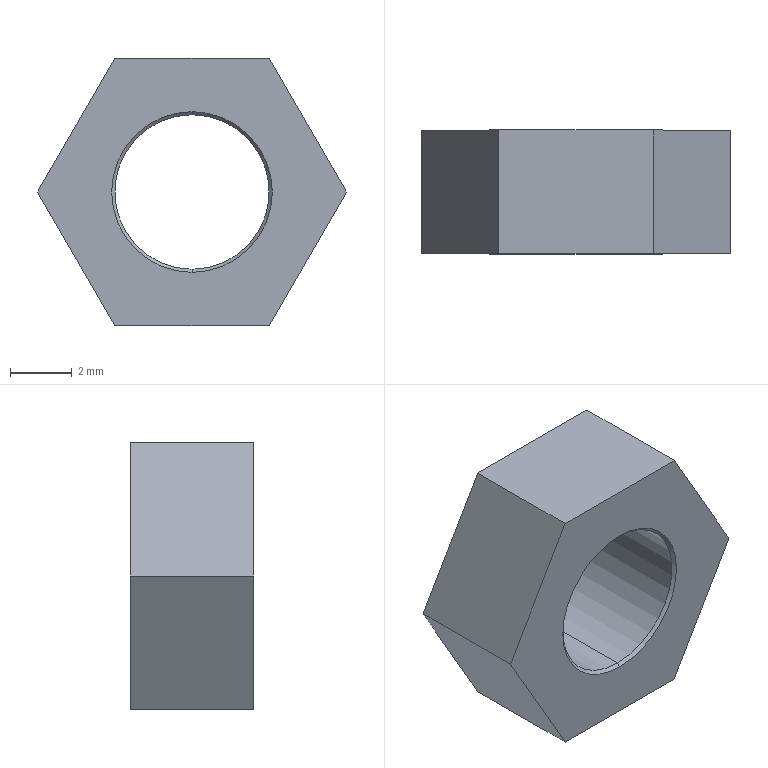Part | SolidWorks | features Chamfer 1, Extrusion 1 | 1 solid | 14 faces | box 10 x 4 x 8.66 mm | volume 181.109 mm3 | plane 8 | cone 4 | cylinder 2 | commonest cylinder face diameters 5 x2
STEP:
#1=CARTESIAN_POINT('',(0.,3.9,-2.5));
#2=VERTEX_POINT('',#1);
#3=CARTESIAN_POINT('',(0.,3.9,2.5));
#4=VERTEX_POINT('',#3);
#5=CARTESIAN_POINT('',(0.,3.9,0.));
#6=DIRECTION('',(0.,1.,0.));
#7=DIRECTION('',(0.,0.,1.));
#8=AXIS2_PLACEMENT_3D('',#5,#6,#7);
#9=CIRCLE('',#8,2.5);
#10=EDGE_CURVE('',#2,#4,#9,.T.);
#11=ORIENTED_EDGE('',*,*,#10,.F.);
#12=CARTESIAN_POINT('',(0.,4.,-2.6));
#13=VERTEX_POINT('',#12);
#14=CARTESIAN_POINT('',(0.,3.9,-2.5));
#15=DIRECTION('',(0.,0.7071,-0.7071));
#16=VECTOR('',#15,1000.);
#17=LINE('',#14,#16);
#18=EDGE_CURVE('',#2,#13,#17,.T.);
#19=ORIENTED_EDGE('',*,*,#18,.T.);
#20=CARTESIAN_POINT('',(0.,4.,2.6));
#21=VERTEX_POINT('',#20);
#22=CARTESIAN_POINT('',(0.,4.,0.));
#23=DIRECTION('',(0.,-1.,0.));
#24=DIRECTION('',(0.,0.,1.));
#25=AXIS2_PLACEMENT_3D('',#22,#23,#24);
#26=CIRCLE('',#25,2.6);
#27=EDGE_CURVE('',#21,#13,#26,.T.);
#28=ORIENTED_EDGE('',*,*,#27,.F.);
#29=CARTESIAN_POINT('',(0.,3.9,2.5));
#30=DIRECTION('',(0.,0.7071,0.7071));
#31=VECTOR('',#30,1000.);
#32=LINE('',#29,#31);
#33=EDGE_CURVE('',#4,#21,#32,.T.);
#34=ORIENTED_EDGE('',*,*,#33,.F.);
#35=EDGE_LOOP('',(#11,#19,#28,#34));
#36=FACE_OUTER_BOUND('',#35,.T.);
#37=CARTESIAN_POINT('',(0.,3.9,0.));
#38=DIRECTION('',(0.,1.,0.));
#39=DIRECTION('',(0.,0.,1.));
#40=AXIS2_PLACEMENT_3D('',#37,#38,#39);
#41=CONICAL_SURFACE('',#40,2.5,0.7854);
#42=ADVANCED_FACE('',(#36),#41,.F.);
#43=CARTESIAN_POINT('',(0.,0.1,2.5));
#44=VERTEX_POINT('',#43);
#45=CARTESIAN_POINT('',(0.,0.1,-2.5));
#46=VERTEX_POINT('',#45);
#47=CARTESIAN_POINT('',(0.,0.1,0.));
#48=DIRECTION('',(0.,-1.,0.));
#49=DIRECTION('',(0.,0.,1.));
#50=AXIS2_PLACEMENT_3D('',#47,#48,#49);
#51=CIRCLE('',#50,2.5);
#52=EDGE_CURVE('',#44,#46,#51,.T.);
#53=ORIENTED_EDGE('',*,*,#52,.F.);
#54=CARTESIAN_POINT('',(0.,0.,2.6));
#55=VERTEX_POINT('',#54);
#56=CARTESIAN_POINT('',(0.,0.,2.6));
#57=DIRECTION('',(0.,-0.7071,0.7071));
#58=VECTOR('',#57,1000.);
#59=LINE('',#56,#58);
#60=EDGE_CURVE('',#44,#55,#59,.T.);
#61=ORIENTED_EDGE('',*,*,#60,.T.);
#62=CARTESIAN_POINT('',(0.,0.,-2.6));
#63=VERTEX_POINT('',#62);
#64=CARTESIAN_POINT('',(0.,0.,0.));
#65=DIRECTION('',(0.,1.,0.));
#66=DIRECTION('',(0.,0.,1.));
#67=AXIS2_PLACEMENT_3D('',#64,#65,#66);
#68=CIRCLE('',#67,2.6);
#69=EDGE_CURVE('',#63,#55,#68,.T.);
#70=ORIENTED_EDGE('',*,*,#69,.F.);
#71=CARTESIAN_POINT('',(0.,0.,-2.6));
#72=DIRECTION('',(0.,-0.7071,-0.7071));
#73=VECTOR('',#72,1000.);
#74=LINE('',#71,#73);
#75=EDGE_CURVE('',#46,#63,#74,.T.);
#76=ORIENTED_EDGE('',*,*,#75,.F.);
#77=EDGE_LOOP('',(#53,#61,#70,#76));
#78=FACE_OUTER_BOUND('',#77,.T.);
#79=CARTESIAN_POINT('',(0.,0.,0.));
#80=DIRECTION('',(0.,-1.,0.));
#81=DIRECTION('',(0.,0.,-1.));
#82=AXIS2_PLACEMENT_3D('',#79,#80,#81);
#83=CONICAL_SURFACE('',#82,2.6,0.7854);
#84=ADVANCED_FACE('',(#78),#83,.F.);
#85=ORIENTED_EDGE('',*,*,#10,.T.);
#86=CARTESIAN_POINT('',(0.,4.,2.5));
#87=DIRECTION('',(0.,-1.,0.));
#88=VECTOR('',#87,1000.);
#89=LINE('',#86,#88);
#90=EDGE_CURVE('',#4,#44,#89,.T.);
#91=ORIENTED_EDGE('',*,*,#90,.T.);
#92=ORIENTED_EDGE('',*,*,#52,.T.);
#93=CARTESIAN_POINT('',(0.,4.,-2.5));
#94=DIRECTION('',(0.,-1.,0.));
#95=VECTOR('',#94,1000.);
#96=LINE('',#93,#95);
#97=EDGE_CURVE('',#2,#46,#96,.T.);
#98=ORIENTED_EDGE('',*,*,#97,.F.);
#99=EDGE_LOOP('',(#85,#91,#92,#98));
#100=FACE_OUTER_BOUND('',#99,.T.);
#101=CARTESIAN_POINT('',(0.,4.,0.));
#102=DIRECTION('',(0.,-1.,0.));
#103=DIRECTION('',(0.,0.,-1.));
#104=AXIS2_PLACEMENT_3D('',#101,#102,#103);
#105=CYLINDRICAL_SURFACE('',#104,2.5);
#106=ADVANCED_FACE('',(#100),#105,.F.);
#107=ORIENTED_EDGE('',*,*,#27,.T.);
#108=CARTESIAN_POINT('',(0.,4.,0.));
#109=DIRECTION('',(0.,-1.,0.));
#110=DIRECTION('',(0.,0.,1.));
#111=AXIS2_PLACEMENT_3D('',#108,#109,#110);
#112=CIRCLE('',#111,2.6);
#113=EDGE_CURVE('',#13,#21,#112,.T.);
#114=ORIENTED_EDGE('',*,*,#113,.T.);
#115=EDGE_LOOP('',(#107,#114));
#116=FACE_BOUND('',#115,.T.);
#117=CARTESIAN_POINT('',(-2.5,4.,4.33));
#118=VERTEX_POINT('',#117);
#119=CARTESIAN_POINT('',(2.5,4.,4.33));
#120=VERTEX_POINT('',#119);
#121=CARTESIAN_POINT('',(-2.5,4.,4.33));
#122=DIRECTION('',(1.,0.,0.));
#123=VECTOR('',#122,1000.);
#124=LINE('',#121,#123);
#125=EDGE_CURVE('',#118,#120,#124,.T.);
#126=ORIENTED_EDGE('',*,*,#125,.T.);
#127=CARTESIAN_POINT('',(5.,4.,0.));
#128=VERTEX_POINT('',#127);
#129=CARTESIAN_POINT('',(2.5,4.,4.33));
#130=DIRECTION('',(0.5,0.,-0.866));
#131=VECTOR('',#130,1000.);
#132=LINE('',#129,#131);
#133=EDGE_CURVE('',#120,#128,#132,.T.);
#134=ORIENTED_EDGE('',*,*,#133,.T.);
#135=CARTESIAN_POINT('',(2.5,4.,-4.33));
#136=VERTEX_POINT('',#135);
#137=CARTESIAN_POINT('',(5.,4.,0.));
#138=DIRECTION('',(-0.5,0.,-0.866));
#139=VECTOR('',#138,1000.);
#140=LINE('',#137,#139);
#141=EDGE_CURVE('',#128,#136,#140,.T.);
#142=ORIENTED_EDGE('',*,*,#141,.T.);
#143=CARTESIAN_POINT('',(-2.5,4.,-4.33));
#144=VERTEX_POINT('',#143);
#145=CARTESIAN_POINT('',(2.5,4.,-4.33));
#146=DIRECTION('',(-1.,0.,0.));
#147=VECTOR('',#146,1000.);
#148=LINE('',#145,#147);
#149=EDGE_CURVE('',#136,#144,#148,.T.);
#150=ORIENTED_EDGE('',*,*,#149,.T.);
#151=CARTESIAN_POINT('',(-5.,4.,0.));
#152=VERTEX_POINT('',#151);
#153=CARTESIAN_POINT('',(-2.5,4.,-4.33));
#154=DIRECTION('',(-0.5,0.,0.866));
#155=VECTOR('',#154,1000.);
#156=LINE('',#153,#155);
#157=EDGE_CURVE('',#144,#152,#156,.T.);
#158=ORIENTED_EDGE('',*,*,#157,.T.);
#159=CARTESIAN_POINT('',(-5.,4.,0.));
#160=DIRECTION('',(0.5,0.,0.866));
#161=VECTOR('',#160,1000.);
#162=LINE('',#159,#161);
#163=EDGE_CURVE('',#152,#118,#162,.T.);
#164=ORIENTED_EDGE('',*,*,#163,.T.);
#165=EDGE_LOOP('',(#126,#134,#142,#150,#158,#164));
#166=FACE_OUTER_BOUND('',#165,.T.);
#167=CARTESIAN_POINT('',(0.,4.,0.));
#168=DIRECTION('',(0.,1.,0.));
#169=DIRECTION('',(0.,0.,1.));
#170=AXIS2_PLACEMENT_3D('',#167,#168,#169);
#171=PLANE('',#170);
#172=ADVANCED_FACE('',(#116,#166),#171,.T.);
#173=ORIENTED_EDGE('',*,*,#69,.T.);
#174=CARTESIAN_POINT('',(0.,0.,0.));
#175=DIRECTION('',(0.,1.,0.));
#176=DIRECTION('',(0.,0.,1.));
#177=AXIS2_PLACEMENT_3D('',#174,#175,#176);
#178=CIRCLE('',#177,2.6);
#179=EDGE_CURVE('',#55,#63,#178,.T.);
#180=ORIENTED_EDGE('',*,*,#179,.T.);
#181=EDGE_LOOP('',(#173,#180));
#182=FACE_BOUND('',#181,.T.);
#183=CARTESIAN_POINT('',(-2.5,0.,4.33));
#184=VERTEX_POINT('',#183);
#185=CARTESIAN_POINT('',(2.5,0.,4.33));
#186=VERTEX_POINT('',#185);
#187=CARTESIAN_POINT('',(-2.5,0.,4.33));
#188=DIRECTION('',(1.,0.,0.));
#189=VECTOR('',#188,1000.);
#190=LINE('',#187,#189);
#191=EDGE_CURVE('',#184,#186,#190,.T.);
#192=ORIENTED_EDGE('',*,*,#191,.F.);
#193=CARTESIAN_POINT('',(-5.,0.,0.));
#194=VERTEX_POINT('',#193);
#195=CARTESIAN_POINT('',(-5.,0.,0.));
#196=DIRECTION('',(0.5,0.,0.866));
#197=VECTOR('',#196,1000.);
#198=LINE('',#195,#197);
#199=EDGE_CURVE('',#194,#184,#198,.T.);
#200=ORIENTED_EDGE('',*,*,#199,.F.);
#201=CARTESIAN_POINT('',(-2.5,0.,-4.33));
#202=VERTEX_POINT('',#201);
#203=CARTESIAN_POINT('',(-2.5,0.,-4.33));
#204=DIRECTION('',(-0.5,0.,0.866));
#205=VECTOR('',#204,1000.);
#206=LINE('',#203,#205);
#207=EDGE_CURVE('',#202,#194,#206,.T.);
#208=ORIENTED_EDGE('',*,*,#207,.F.);
#209=CARTESIAN_POINT('',(2.5,0.,-4.33));
#210=VERTEX_POINT('',#209);
#211=CARTESIAN_POINT('',(2.5,0.,-4.33));
#212=DIRECTION('',(-1.,0.,0.));
#213=VECTOR('',#212,1000.);
#214=LINE('',#211,#213);
#215=EDGE_CURVE('',#210,#202,#214,.T.);
#216=ORIENTED_EDGE('',*,*,#215,.F.);
#217=CARTESIAN_POINT('',(5.,0.,0.));
#218=VERTEX_POINT('',#217);
#219=CARTESIAN_POINT('',(5.,0.,0.));
#220=DIRECTION('',(-0.5,0.,-0.866));
#221=VECTOR('',#220,1000.);
#222=LINE('',#219,#221);
#223=EDGE_CURVE('',#218,#210,#222,.T.);
#224=ORIENTED_EDGE('',*,*,#223,.F.);
#225=CARTESIAN_POINT('',(2.5,0.,4.33));
#226=DIRECTION('',(0.5,0.,-0.866));
#227=VECTOR('',#226,1000.);
#228=LINE('',#225,#227);
#229=EDGE_CURVE('',#186,#218,#228,.T.);
#230=ORIENTED_EDGE('',*,*,#229,.F.);
#231=EDGE_LOOP('',(#192,#200,#208,#216,#224,#230));
#232=FACE_OUTER_BOUND('',#231,.T.);
#233=CARTESIAN_POINT('',(0.,0.,0.));
#234=DIRECTION('',(0.,1.,0.));
#235=DIRECTION('',(0.,0.,1.));
#236=AXIS2_PLACEMENT_3D('',#233,#234,#235);
#237=PLANE('',#236);
#238=ADVANCED_FACE('',(#182,#232),#237,.F.);
#239=ORIENTED_EDGE('',*,*,#191,.T.);
#240=CARTESIAN_POINT('',(2.5,4.,4.33));
#241=DIRECTION('',(0.,-1.,0.));
#242=VECTOR('',#241,1000.);
#243=LINE('',#240,#242);
#244=EDGE_CURVE('',#120,#186,#243,.T.);
#245=ORIENTED_EDGE('',*,*,#244,.F.);
#246=ORIENTED_EDGE('',*,*,#125,.F.);
#247=CARTESIAN_POINT('',(-2.5,4.,4.33));
#248=DIRECTION('',(0.,-1.,0.));
#249=VECTOR('',#248,1000.);
#250=LINE('',#247,#249);
#251=EDGE_CURVE('',#118,#184,#250,.T.);
#252=ORIENTED_EDGE('',*,*,#251,.T.);
#253=EDGE_LOOP('',(#239,#245,#246,#252));
#254=FACE_OUTER_BOUND('',#253,.T.);
#255=CARTESIAN_POINT('',(-2.5,4.,4.33));
#256=DIRECTION('',(0.,0.,-1.));
#257=DIRECTION('',(-1.,0.,0.));
#258=AXIS2_PLACEMENT_3D('',#255,#256,#257);
#259=PLANE('',#258);
#260=ADVANCED_FACE('',(#254),#259,.F.);
#261=ORIENTED_EDGE('',*,*,#229,.T.);
#262=CARTESIAN_POINT('',(5.,4.,0.));
#263=DIRECTION('',(0.,-1.,0.));
#264=VECTOR('',#263,1000.);
#265=LINE('',#262,#264);
#266=EDGE_CURVE('',#128,#218,#265,.T.);
#267=ORIENTED_EDGE('',*,*,#266,.F.);
#268=ORIENTED_EDGE('',*,*,#133,.F.);
#269=ORIENTED_EDGE('',*,*,#244,.T.);
#270=EDGE_LOOP('',(#261,#267,#268,#269));
#271=FACE_OUTER_BOUND('',#270,.T.);
#272=CARTESIAN_POINT('',(2.5,4.,4.33));
#273=DIRECTION('',(-0.866,0.,-0.5));
#274=DIRECTION('',(-0.5,0.,0.866));
#275=AXIS2_PLACEMENT_3D('',#272,#273,#274);
#276=PLANE('',#275);
#277=ADVANCED_FACE('',(#271),#276,.F.);
#278=ORIENTED_EDGE('',*,*,#223,.T.);
#279=CARTESIAN_POINT('',(2.5,4.,-4.33));
#280=DIRECTION('',(0.,-1.,0.));
#281=VECTOR('',#280,1000.);
#282=LINE('',#279,#281);
#283=EDGE_CURVE('',#136,#210,#282,.T.);
#284=ORIENTED_EDGE('',*,*,#283,.F.);
#285=ORIENTED_EDGE('',*,*,#141,.F.);
#286=ORIENTED_EDGE('',*,*,#266,.T.);
#287=EDGE_LOOP('',(#278,#284,#285,#286));
#288=FACE_OUTER_BOUND('',#287,.T.);
#289=CARTESIAN_POINT('',(5.,4.,0.));
#290=DIRECTION('',(-0.866,0.,0.5));
#291=DIRECTION('',(0.5,0.,0.866));
#292=AXIS2_PLACEMENT_3D('',#289,#290,#291);
#293=PLANE('',#292);
#294=ADVANCED_FACE('',(#288),#293,.F.);
#295=ORIENTED_EDGE('',*,*,#215,.T.);
#296=CARTESIAN_POINT('',(-2.5,4.,-4.33));
#297=DIRECTION('',(0.,-1.,0.));
#298=VECTOR('',#297,1000.);
#299=LINE('',#296,#298);
#300=EDGE_CURVE('',#144,#202,#299,.T.);
#301=ORIENTED_EDGE('',*,*,#300,.F.);
#302=ORIENTED_EDGE('',*,*,#149,.F.);
#303=ORIENTED_EDGE('',*,*,#283,.T.);
#304=EDGE_LOOP('',(#295,#301,#302,#303));
#305=FACE_OUTER_BOUND('',#304,.T.);
#306=CARTESIAN_POINT('',(2.5,4.,-4.33));
#307=DIRECTION('',(0.,0.,1.));
#308=DIRECTION('',(1.,0.,0.));
#309=AXIS2_PLACEMENT_3D('',#306,#307,#308);
#310=PLANE('',#309);
#311=ADVANCED_FACE('',(#305),#310,.F.);
#312=ORIENTED_EDGE('',*,*,#207,.T.);
#313=CARTESIAN_POINT('',(-5.,4.,0.));
#314=DIRECTION('',(0.,-1.,0.));
#315=VECTOR('',#314,1000.);
#316=LINE('',#313,#315);
#317=EDGE_CURVE('',#152,#194,#316,.T.);
#318=ORIENTED_EDGE('',*,*,#317,.F.);
#319=ORIENTED_EDGE('',*,*,#157,.F.);
#320=ORIENTED_EDGE('',*,*,#300,.T.);
#321=EDGE_LOOP('',(#312,#318,#319,#320));
#322=FACE_OUTER_BOUND('',#321,.T.);
#323=CARTESIAN_POINT('',(-2.5,4.,-4.33));
#324=DIRECTION('',(0.866,0.,0.5));
#325=DIRECTION('',(0.5,0.,-0.866));
#326=AXIS2_PLACEMENT_3D('',#323,#324,#325);
#327=PLANE('',#326);
#328=ADVANCED_FACE('',(#322),#327,.F.);
#329=ORIENTED_EDGE('',*,*,#199,.T.);
#330=ORIENTED_EDGE('',*,*,#251,.F.);
#331=ORIENTED_EDGE('',*,*,#163,.F.);
#332=ORIENTED_EDGE('',*,*,#317,.T.);
#333=EDGE_LOOP('',(#329,#330,#331,#332));
#334=FACE_OUTER_BOUND('',#333,.T.);
#335=CARTESIAN_POINT('',(-5.,4.,0.));
#336=DIRECTION('',(0.866,0.,-0.5));
#337=DIRECTION('',(-0.5,0.,-0.866));
#338=AXIS2_PLACEMENT_3D('',#335,#336,#337);
#339=PLANE('',#338);
#340=ADVANCED_FACE('',(#334),#339,.F.);
#341=ORIENTED_EDGE('',*,*,#90,.F.);
#342=CARTESIAN_POINT('',(0.,3.9,0.));
#343=DIRECTION('',(0.,1.,0.));
#344=DIRECTION('',(0.,0.,1.));
#345=AXIS2_PLACEMENT_3D('',#342,#343,#344);
#346=CIRCLE('',#345,2.5);
#347=EDGE_CURVE('',#4,#2,#346,.T.);
#348=ORIENTED_EDGE('',*,*,#347,.T.);
#349=ORIENTED_EDGE('',*,*,#97,.T.);
#350=CARTESIAN_POINT('',(0.,0.1,0.));
#351=DIRECTION('',(0.,-1.,0.));
#352=DIRECTION('',(0.,0.,1.));
#353=AXIS2_PLACEMENT_3D('',#350,#351,#352);
#354=CIRCLE('',#353,2.5);
#355=EDGE_CURVE('',#46,#44,#354,.T.);
#356=ORIENTED_EDGE('',*,*,#355,.T.);
#357=EDGE_LOOP('',(#341,#348,#349,#356));
#358=FACE_OUTER_BOUND('',#357,.T.);
#359=CARTESIAN_POINT('',(0.,4.,0.));
#360=DIRECTION('',(0.,-1.,0.));
#361=DIRECTION('',(0.,0.,-1.));
#362=AXIS2_PLACEMENT_3D('',#359,#360,#361);
#363=CYLINDRICAL_SURFACE('',#362,2.5);
#364=ADVANCED_FACE('',(#358),#363,.F.);
#365=ORIENTED_EDGE('',*,*,#60,.F.);
#366=ORIENTED_EDGE('',*,*,#355,.F.);
#367=ORIENTED_EDGE('',*,*,#75,.T.);
#368=ORIENTED_EDGE('',*,*,#179,.F.);
#369=EDGE_LOOP('',(#365,#366,#367,#368));
#370=FACE_OUTER_BOUND('',#369,.T.);
#371=CARTESIAN_POINT('',(0.,0.,0.));
#372=DIRECTION('',(0.,-1.,0.));
#373=DIRECTION('',(0.,0.,-1.));
#374=AXIS2_PLACEMENT_3D('',#371,#372,#373);
#375=CONICAL_SURFACE('',#374,2.6,0.7854);
#376=ADVANCED_FACE('',(#370),#375,.F.);
#377=ORIENTED_EDGE('',*,*,#18,.F.);
#378=ORIENTED_EDGE('',*,*,#347,.F.);
#379=ORIENTED_EDGE('',*,*,#33,.T.);
#380=ORIENTED_EDGE('',*,*,#113,.F.);
#381=EDGE_LOOP('',(#377,#378,#379,#380));
#382=FACE_OUTER_BOUND('',#381,.T.);
#383=CARTESIAN_POINT('',(0.,3.9,0.));
#384=DIRECTION('',(0.,1.,0.));
#385=DIRECTION('',(0.,0.,1.));
#386=AXIS2_PLACEMENT_3D('',#383,#384,#385);
#387=CONICAL_SURFACE('',#386,2.5,0.7854);
#388=ADVANCED_FACE('',(#382),#387,.F.);
#389=CLOSED_SHELL('',(#42,#84,#106,#172,#238,#260,#277,#294,#311,#328,#340,#364,#376,#388));
#390=MANIFOLD_SOLID_BREP('',#389);
#391=CARTESIAN_POINT('',(0.,0.,0.));
#392=DIRECTION('',(0.,0.,1.));
#393=DIRECTION('',(1.,0.,0.));
#394=AXIS2_PLACEMENT_3D('',#391,#392,#393);
#395=(LENGTH_UNIT()NAMED_UNIT(*)SI_UNIT(.MILLI.,.METRE.));
#396=UNCERTAINTY_MEASURE_WITH_UNIT(LENGTH_MEASURE(0.00001),#395,'','');
#397=(NAMED_UNIT(*)PLANE_ANGLE_UNIT()SI_UNIT($,.RADIAN.));
#398=(NAMED_UNIT(*)SI_UNIT($,.STERADIAN.)SOLID_ANGLE_UNIT());
#399=(GEOMETRIC_REPRESENTATION_CONTEXT(3)GLOBAL_UNCERTAINTY_ASSIGNED_CONTEXT((#396))GLOBAL_UNIT_ASSIGNED_CONTEXT((#395,#397,#398))REPRESENTATION_CONTEXT('',''));
#400=ADVANCED_BREP_SHAPE_REPRESENTATION('',(#390,#394),#399);